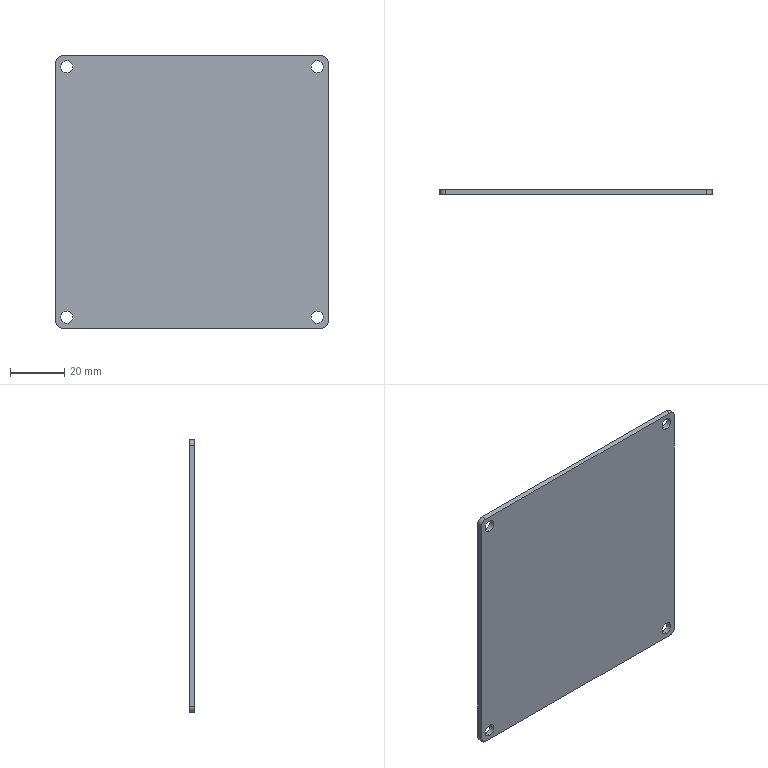Part | STEP file | 护Plate 3 | 1 solid | 18 faces | box 100 x 2 x 100 mm | volume 19866 mm3 | cylinder 12 | plane 6 | commonest cylinder face diameters 4.5 x8 4 x4